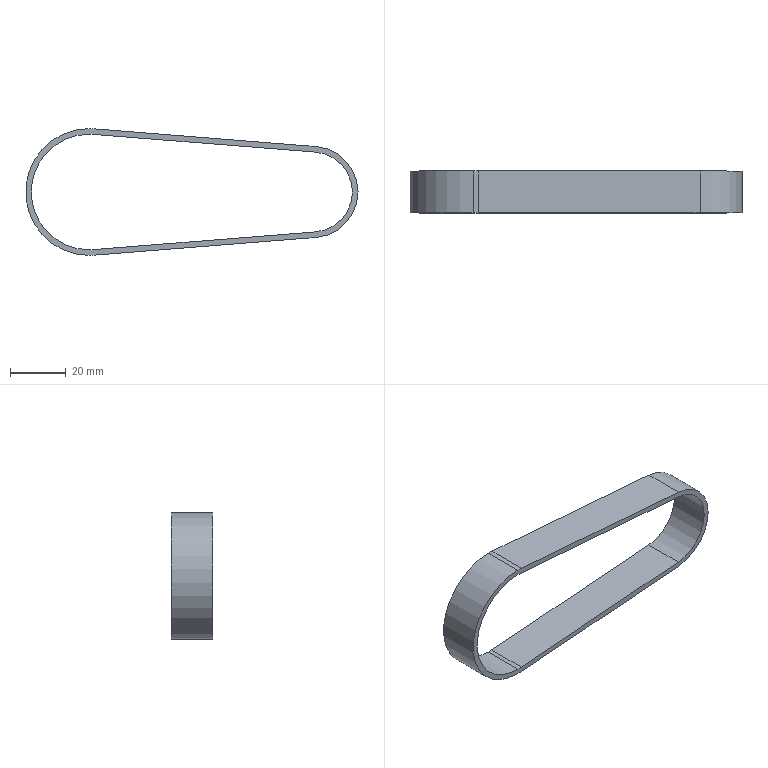Part | STEP file | Timing Belt 270-5M-15mm Wide | 1 solid | 14 faces | box 119.02 x 15 x 45.38 mm | volume 8304 mm3 | cylinder 8 | plane 6 | commonest cylinder face diameters 41.38 x3 45.38 x3 28.66 x1 32.66 x1
STEP:
#1=CARTESIAN_POINT('',(0.,0.,0.));
#2=DIRECTION('',(0.,0.,1.));
#3=DIRECTION('',(1.,0.,0.));
#4=AXIS2_PLACEMENT_3D('',#1,#2,#3);
#5=CARTESIAN_POINT('',(0.,7.5,-20.69));
#6=VERTEX_POINT('',#5);
#7=CARTESIAN_POINT('',(0.,-7.5,-20.69));
#8=VERTEX_POINT('',#7);
#9=CARTESIAN_POINT('',(0.,7.5,-20.69));
#10=DIRECTION('',(0.,-1.,0.));
#11=VECTOR('',#10,1.);
#12=LINE('',#9,#11);
#13=CARTESIAN_POINT('',(0.,7.5,0.));
#14=DIRECTION('',(0.,-1.,0.));
#15=DIRECTION('',(0.,0.,-1.));
#16=AXIS2_PLACEMENT_3D('',#13,#14,#15);
#17=CYLINDRICAL_SURFACE('',#16,20.69);
#18=CARTESIAN_POINT('',(6.283,0.));
#19=DIRECTION('',(0.,1.));
#20=VECTOR('',#19,1.);
#21=LINE('',#18,#20);
#22=(GEOMETRIC_REPRESENTATION_CONTEXT(2)PARAMETRIC_REPRESENTATION_CONTEXT()REPRESENTATION_CONTEXT('',''));
#23=DEFINITIONAL_REPRESENTATION('',(#21),#22);
#24=PCURVE('',#17,#23);
#25=CARTESIAN_POINT('',(0.,7.5,0.));
#26=DIRECTION('',(0.,-1.,0.));
#27=DIRECTION('',(0.,0.,-1.));
#28=AXIS2_PLACEMENT_3D('',#25,#26,#27);
#29=CYLINDRICAL_SURFACE('',#28,20.69);
#30=CARTESIAN_POINT('',(0.,0.));
#31=DIRECTION('',(0.,1.));
#32=VECTOR('',#31,1.);
#33=LINE('',#30,#32);
#34=(GEOMETRIC_REPRESENTATION_CONTEXT(2)PARAMETRIC_REPRESENTATION_CONTEXT()REPRESENTATION_CONTEXT('',''));
#35=DEFINITIONAL_REPRESENTATION('',(#33),#34);
#36=PCURVE('',#29,#35);
#37=SURFACE_CURVE('',#12,(#24,#36),.PCURVE_S1.);
#38=EDGE_CURVE('',#6,#8,#37,.T.);
#39=ORIENTED_EDGE('',*,*,#38,.T.);
#40=CARTESIAN_POINT('',(0.,-7.5,20.69));
#41=VERTEX_POINT('',#40);
#42=CARTESIAN_POINT('',(0.,-7.5,0.));
#43=DIRECTION('',(0.,1.,0.));
#44=DIRECTION('',(0.,0.,1.));
#45=AXIS2_PLACEMENT_3D('',#42,#43,#44);
#46=CIRCLE('',#45,20.69);
#47=CARTESIAN_POINT('',(9.425,15.));
#48=DIRECTION('',(-1.,0.));
#49=VECTOR('',#48,1.);
#50=LINE('',#47,#49);
#51=(GEOMETRIC_REPRESENTATION_CONTEXT(2)PARAMETRIC_REPRESENTATION_CONTEXT()REPRESENTATION_CONTEXT('',''));
#52=DEFINITIONAL_REPRESENTATION('',(#50),#51);
#53=PCURVE('',#17,#52);
#54=CARTESIAN_POINT('',(80.,-7.5,0.));
#55=DIRECTION('',(0.,1.,0.));
#56=DIRECTION('',(0.,0.,1.));
#57=AXIS2_PLACEMENT_3D('',#54,#55,#56);
#58=PLANE('',#57);
#59=CARTESIAN_POINT('',(0.,-80.));
#60=DIRECTION('',(1.,0.));
#61=AXIS2_PLACEMENT_2D('',#59,#60);
#62=CIRCLE('',#61,20.69);
#63=(GEOMETRIC_REPRESENTATION_CONTEXT(2)PARAMETRIC_REPRESENTATION_CONTEXT()REPRESENTATION_CONTEXT('',''));
#64=DEFINITIONAL_REPRESENTATION('',(#62),#63);
#65=PCURVE('',#58,#64);
#66=SURFACE_CURVE('',#46,(#53,#65),.PCURVE_S1.);
#67=EDGE_CURVE('',#8,#41,#66,.T.);
#68=ORIENTED_EDGE('',*,*,#67,.T.);
#69=CARTESIAN_POINT('',(0.,7.5,20.69));
#70=VERTEX_POINT('',#69);
#71=CARTESIAN_POINT('',(0.,7.5,20.69));
#72=DIRECTION('',(0.,-1.,0.));
#73=VECTOR('',#72,1.);
#74=LINE('',#71,#73);
#75=CARTESIAN_POINT('',(3.142,0.));
#76=DIRECTION('',(0.,1.));
#77=VECTOR('',#76,1.);
#78=LINE('',#75,#77);
#79=(GEOMETRIC_REPRESENTATION_CONTEXT(2)PARAMETRIC_REPRESENTATION_CONTEXT()REPRESENTATION_CONTEXT('',''));
#80=DEFINITIONAL_REPRESENTATION('',(#78),#79);
#81=PCURVE('',#17,#80);
#82=CARTESIAN_POINT('',(0.,7.5,0.));
#83=DIRECTION('',(0.,-1.,0.));
#84=DIRECTION('',(0.,0.,-1.));
#85=AXIS2_PLACEMENT_3D('',#82,#83,#84);
#86=CYLINDRICAL_SURFACE('',#85,20.69);
#87=CARTESIAN_POINT('',(3.142,0.));
#88=DIRECTION('',(0.,1.));
#89=VECTOR('',#88,1.);
#90=LINE('',#87,#89);
#91=(GEOMETRIC_REPRESENTATION_CONTEXT(2)PARAMETRIC_REPRESENTATION_CONTEXT()REPRESENTATION_CONTEXT('',''));
#92=DEFINITIONAL_REPRESENTATION('',(#90),#91);
#93=PCURVE('',#86,#92);
#94=SURFACE_CURVE('',#74,(#81,#93),.PCURVE_S1.);
#95=EDGE_CURVE('',#70,#41,#94,.T.);
#96=ORIENTED_EDGE('',*,*,#95,.F.);
#97=CARTESIAN_POINT('',(0.,7.5,0.));
#98=DIRECTION('',(0.,1.,0.));
#99=DIRECTION('',(0.,0.,1.));
#100=AXIS2_PLACEMENT_3D('',#97,#98,#99);
#101=CIRCLE('',#100,20.69);
#102=CARTESIAN_POINT('',(9.425,0.));
#103=DIRECTION('',(-1.,0.));
#104=VECTOR('',#103,1.);
#105=LINE('',#102,#104);
#106=(GEOMETRIC_REPRESENTATION_CONTEXT(2)PARAMETRIC_REPRESENTATION_CONTEXT()REPRESENTATION_CONTEXT('',''));
#107=DEFINITIONAL_REPRESENTATION('',(#105),#106);
#108=PCURVE('',#17,#107);
#109=CARTESIAN_POINT('',(80.,7.5,0.));
#110=DIRECTION('',(0.,1.,0.));
#111=DIRECTION('',(0.,0.,1.));
#112=AXIS2_PLACEMENT_3D('',#109,#110,#111);
#113=PLANE('',#112);
#114=CARTESIAN_POINT('',(0.,-80.));
#115=DIRECTION('',(1.,0.));
#116=AXIS2_PLACEMENT_2D('',#114,#115);
#117=CIRCLE('',#116,20.69);
#118=(GEOMETRIC_REPRESENTATION_CONTEXT(2)PARAMETRIC_REPRESENTATION_CONTEXT()REPRESENTATION_CONTEXT('',''));
#119=DEFINITIONAL_REPRESENTATION('',(#117),#118);
#120=PCURVE('',#113,#119);
#121=SURFACE_CURVE('',#101,(#108,#120),.PCURVE_S1.);
#122=EDGE_CURVE('',#6,#70,#121,.T.);
#123=ORIENTED_EDGE('',*,*,#122,.F.);
#124=EDGE_LOOP('',(#39,#68,#96,#123));
#125=FACE_BOUND('',#124,.F.);
#126=ADVANCED_FACE('',(#125),#17,.F.);
#127=CARTESIAN_POINT('',(1.645,7.5,-20.625));
#128=VERTEX_POINT('',#127);
#129=CARTESIAN_POINT('',(1.645,-7.5,-20.625));
#130=VERTEX_POINT('',#129);
#131=CARTESIAN_POINT('',(1.645,7.5,-20.625));
#132=DIRECTION('',(0.,-1.,0.));
#133=VECTOR('',#132,1.);
#134=LINE('',#131,#133);
#135=CARTESIAN_POINT('',(0.07958,0.));
#136=DIRECTION('',(0.,1.));
#137=VECTOR('',#136,1.);
#138=LINE('',#135,#137);
#139=(GEOMETRIC_REPRESENTATION_CONTEXT(2)PARAMETRIC_REPRESENTATION_CONTEXT()REPRESENTATION_CONTEXT('',''));
#140=DEFINITIONAL_REPRESENTATION('',(#138),#139);
#141=PCURVE('',#29,#140);
#142=CARTESIAN_POINT('',(1.645,7.5,-20.625));
#143=DIRECTION('',(-0.0795,0.,0.9968));
#144=DIRECTION('',(0.9968,0.,0.0795));
#145=AXIS2_PLACEMENT_3D('',#142,#143,#144);
#146=PLANE('',#145);
#147=CARTESIAN_POINT('',(0.,0.));
#148=DIRECTION('',(0.,-1.));
#149=VECTOR('',#148,1.);
#150=LINE('',#147,#149);
#151=(GEOMETRIC_REPRESENTATION_CONTEXT(2)PARAMETRIC_REPRESENTATION_CONTEXT()REPRESENTATION_CONTEXT('',''));
#152=DEFINITIONAL_REPRESENTATION('',(#150),#151);
#153=PCURVE('',#146,#152);
#154=SURFACE_CURVE('',#134,(#141,#153),.PCURVE_S1.);
#155=EDGE_CURVE('',#128,#130,#154,.T.);
#156=ORIENTED_EDGE('',*,*,#155,.T.);
#157=CARTESIAN_POINT('',(0.,-7.5,0.));
#158=DIRECTION('',(0.,1.,0.));
#159=DIRECTION('',(0.,0.,1.));
#160=AXIS2_PLACEMENT_3D('',#157,#158,#159);
#161=CIRCLE('',#160,20.69);
#162=CARTESIAN_POINT('',(3.142,15.));
#163=DIRECTION('',(-1.,0.));
#164=VECTOR('',#163,1.);
#165=LINE('',#162,#164);
#166=(GEOMETRIC_REPRESENTATION_CONTEXT(2)PARAMETRIC_REPRESENTATION_CONTEXT()REPRESENTATION_CONTEXT('',''));
#167=DEFINITIONAL_REPRESENTATION('',(#165),#166);
#168=PCURVE('',#29,#167);
#169=CARTESIAN_POINT('',(0.,-80.));
#170=DIRECTION('',(1.,0.));
#171=AXIS2_PLACEMENT_2D('',#169,#170);
#172=CIRCLE('',#171,20.69);
#173=(GEOMETRIC_REPRESENTATION_CONTEXT(2)PARAMETRIC_REPRESENTATION_CONTEXT()REPRESENTATION_CONTEXT('',''));
#174=DEFINITIONAL_REPRESENTATION('',(#172),#173);
#175=PCURVE('',#58,#174);
#176=SURFACE_CURVE('',#161,(#168,#175),.PCURVE_S1.);
#177=EDGE_CURVE('',#130,#8,#176,.T.);
#178=ORIENTED_EDGE('',*,*,#177,.T.);
#179=ORIENTED_EDGE('',*,*,#38,.F.);
#180=CARTESIAN_POINT('',(0.,7.5,0.));
#181=DIRECTION('',(0.,1.,0.));
#182=DIRECTION('',(0.,0.,1.));
#183=AXIS2_PLACEMENT_3D('',#180,#181,#182);
#184=CIRCLE('',#183,20.69);
#185=CARTESIAN_POINT('',(3.142,0.));
#186=DIRECTION('',(-1.,0.));
#187=VECTOR('',#186,1.);
#188=LINE('',#185,#187);
#189=(GEOMETRIC_REPRESENTATION_CONTEXT(2)PARAMETRIC_REPRESENTATION_CONTEXT()REPRESENTATION_CONTEXT('',''));
#190=DEFINITIONAL_REPRESENTATION('',(#188),#189);
#191=PCURVE('',#29,#190);
#192=CARTESIAN_POINT('',(0.,-80.));
#193=DIRECTION('',(1.,0.));
#194=AXIS2_PLACEMENT_2D('',#192,#193);
#195=CIRCLE('',#194,20.69);
#196=(GEOMETRIC_REPRESENTATION_CONTEXT(2)PARAMETRIC_REPRESENTATION_CONTEXT()REPRESENTATION_CONTEXT('',''));
#197=DEFINITIONAL_REPRESENTATION('',(#195),#196);
#198=PCURVE('',#113,#197);
#199=SURFACE_CURVE('',#184,(#191,#198),.PCURVE_S1.);
#200=EDGE_CURVE('',#128,#6,#199,.T.);
#201=ORIENTED_EDGE('',*,*,#200,.F.);
#202=EDGE_LOOP('',(#156,#178,#179,#201));
#203=FACE_BOUND('',#202,.F.);
#204=ADVANCED_FACE('',(#203),#29,.F.);
#205=CARTESIAN_POINT('',(0.,7.5,22.69));
#206=VERTEX_POINT('',#205);
#207=CARTESIAN_POINT('',(1.804,7.5,22.618));
#208=VERTEX_POINT('',#207);
#209=CARTESIAN_POINT('',(0.,7.5,0.));
#210=DIRECTION('',(0.,1.,0.));
#211=DIRECTION('',(1.,0.,0.));
#212=AXIS2_PLACEMENT_3D('',#209,#210,#211);
#213=CIRCLE('',#212,22.69);
#214=CARTESIAN_POINT('',(0.,7.5,0.));
#215=DIRECTION('',(0.,-1.,0.));
#216=DIRECTION('',(0.,0.,-1.));
#217=AXIS2_PLACEMENT_3D('',#214,#215,#216);
#218=CYLINDRICAL_SURFACE('',#217,22.69);
#219=CARTESIAN_POINT('',(7.854,0.));
#220=DIRECTION('',(-1.,0.));
#221=VECTOR('',#220,1.);
#222=LINE('',#219,#221);
#223=(GEOMETRIC_REPRESENTATION_CONTEXT(2)PARAMETRIC_REPRESENTATION_CONTEXT()REPRESENTATION_CONTEXT('',''));
#224=DEFINITIONAL_REPRESENTATION('',(#222),#223);
#225=PCURVE('',#218,#224);
#226=CARTESIAN_POINT('',(0.,-80.));
#227=DIRECTION('',(0.,1.));
#228=AXIS2_PLACEMENT_2D('',#226,#227);
#229=CIRCLE('',#228,22.69);
#230=(GEOMETRIC_REPRESENTATION_CONTEXT(2)PARAMETRIC_REPRESENTATION_CONTEXT()REPRESENTATION_CONTEXT('',''));
#231=DEFINITIONAL_REPRESENTATION('',(#229),#230);
#232=PCURVE('',#113,#231);
#233=SURFACE_CURVE('',#213,(#225,#232),.PCURVE_S1.);
#234=EDGE_CURVE('',#206,#208,#233,.T.);
#235=ORIENTED_EDGE('',*,*,#234,.F.);
#236=CARTESIAN_POINT('',(0.,-7.5,22.69));
#237=VERTEX_POINT('',#236);
#238=CARTESIAN_POINT('',(0.,7.5,22.69));
#239=DIRECTION('',(0.,-1.,0.));
#240=VECTOR('',#239,1.);
#241=LINE('',#238,#240);
#242=CARTESIAN_POINT('',(3.142,0.));
#243=DIRECTION('',(0.,1.));
#244=VECTOR('',#243,1.);
#245=LINE('',#242,#244);
#246=(GEOMETRIC_REPRESENTATION_CONTEXT(2)PARAMETRIC_REPRESENTATION_CONTEXT()REPRESENTATION_CONTEXT('',''));
#247=DEFINITIONAL_REPRESENTATION('',(#245),#246);
#248=PCURVE('',#218,#247);
#249=CARTESIAN_POINT('',(0.,7.5,0.));
#250=DIRECTION('',(0.,-1.,0.));
#251=DIRECTION('',(0.,0.,-1.));
#252=AXIS2_PLACEMENT_3D('',#249,#250,#251);
#253=CYLINDRICAL_SURFACE('',#252,22.69);
#254=CARTESIAN_POINT('',(3.142,0.));
#255=DIRECTION('',(0.,1.));
#256=VECTOR('',#255,1.);
#257=LINE('',#254,#256);
#258=(GEOMETRIC_REPRESENTATION_CONTEXT(2)PARAMETRIC_REPRESENTATION_CONTEXT()REPRESENTATION_CONTEXT('',''));
#259=DEFINITIONAL_REPRESENTATION('',(#257),#258);
#260=PCURVE('',#253,#259);
#261=SURFACE_CURVE('',#241,(#248,#260),.PCURVE_S1.);
#262=EDGE_CURVE('',#206,#237,#261,.T.);
#263=ORIENTED_EDGE('',*,*,#262,.T.);
#264=CARTESIAN_POINT('',(1.804,-7.5,22.618));
#265=VERTEX_POINT('',#264);
#266=CARTESIAN_POINT('',(0.,-7.5,0.));
#267=DIRECTION('',(0.,1.,0.));
#268=DIRECTION('',(1.,0.,0.));
#269=AXIS2_PLACEMENT_3D('',#266,#267,#268);
#270=CIRCLE('',#269,22.69);
#271=CARTESIAN_POINT('',(7.854,15.));
#272=DIRECTION('',(-1.,0.));
#273=VECTOR('',#272,1.);
#274=LINE('',#271,#273);
#275=(GEOMETRIC_REPRESENTATION_CONTEXT(2)PARAMETRIC_REPRESENTATION_CONTEXT()REPRESENTATION_CONTEXT('',''));
#276=DEFINITIONAL_REPRESENTATION('',(#274),#275);
#277=PCURVE('',#218,#276);
#278=CARTESIAN_POINT('',(0.,-80.));
#279=DIRECTION('',(0.,1.));
#280=AXIS2_PLACEMENT_2D('',#278,#279);
#281=CIRCLE('',#280,22.69);
#282=(GEOMETRIC_REPRESENTATION_CONTEXT(2)PARAMETRIC_REPRESENTATION_CONTEXT()REPRESENTATION_CONTEXT('',''));
#283=DEFINITIONAL_REPRESENTATION('',(#281),#282);
#284=PCURVE('',#58,#283);
#285=SURFACE_CURVE('',#270,(#277,#284),.PCURVE_S1.);
#286=EDGE_CURVE('',#237,#265,#285,.T.);
#287=ORIENTED_EDGE('',*,*,#286,.T.);
#288=CARTESIAN_POINT('',(1.804,7.5,22.618));
#289=DIRECTION('',(0.,-1.,0.));
#290=VECTOR('',#289,1.);
#291=LINE('',#288,#290);
#292=CARTESIAN_POINT('',(3.062,0.));
#293=DIRECTION('',(0.,1.));
#294=VECTOR('',#293,1.);
#295=LINE('',#292,#294);
#296=(GEOMETRIC_REPRESENTATION_CONTEXT(2)PARAMETRIC_REPRESENTATION_CONTEXT()REPRESENTATION_CONTEXT('',''));
#297=DEFINITIONAL_REPRESENTATION('',(#295),#296);
#298=PCURVE('',#218,#297);
#299=CARTESIAN_POINT('',(1.804,7.5,22.618));
#300=DIRECTION('',(-0.0795,0.,-0.9968));
#301=DIRECTION('',(-0.9968,0.,0.0795));
#302=AXIS2_PLACEMENT_3D('',#299,#300,#301);
#303=PLANE('',#302);
#304=CARTESIAN_POINT('',(0.,0.));
#305=DIRECTION('',(0.,-1.));
#306=VECTOR('',#305,1.);
#307=LINE('',#304,#306);
#308=(GEOMETRIC_REPRESENTATION_CONTEXT(2)PARAMETRIC_REPRESENTATION_CONTEXT()REPRESENTATION_CONTEXT('',''));
#309=DEFINITIONAL_REPRESENTATION('',(#307),#308);
#310=PCURVE('',#303,#309);
#311=SURFACE_CURVE('',#291,(#298,#310),.PCURVE_S1.);
#312=EDGE_CURVE('',#208,#265,#311,.T.);
#313=ORIENTED_EDGE('',*,*,#312,.F.);
#314=EDGE_LOOP('',(#235,#263,#287,#313));
#315=FACE_BOUND('',#314,.T.);
#316=ADVANCED_FACE('',(#315),#218,.T.);
#317=ORIENTED_EDGE('',*,*,#262,.F.);
#318=CARTESIAN_POINT('',(0.,7.5,-22.69));
#319=VERTEX_POINT('',#318);
#320=CARTESIAN_POINT('',(0.,7.5,0.));
#321=DIRECTION('',(0.,1.,0.));
#322=DIRECTION('',(1.,0.,0.));
#323=AXIS2_PLACEMENT_3D('',#320,#321,#322);
#324=CIRCLE('',#323,22.69);
#325=CARTESIAN_POINT('',(7.854,0.));
#326=DIRECTION('',(-1.,0.));
#327=VECTOR('',#326,1.);
#328=LINE('',#325,#327);
#329=(GEOMETRIC_REPRESENTATION_CONTEXT(2)PARAMETRIC_REPRESENTATION_CONTEXT()REPRESENTATION_CONTEXT('',''));
#330=DEFINITIONAL_REPRESENTATION('',(#328),#329);
#331=PCURVE('',#253,#330);
#332=CARTESIAN_POINT('',(0.,-80.));
#333=DIRECTION('',(0.,1.));
#334=AXIS2_PLACEMENT_2D('',#332,#333);
#335=CIRCLE('',#334,22.69);
#336=(GEOMETRIC_REPRESENTATION_CONTEXT(2)PARAMETRIC_REPRESENTATION_CONTEXT()REPRESENTATION_CONTEXT('',''));
#337=DEFINITIONAL_REPRESENTATION('',(#335),#336);
#338=PCURVE('',#113,#337);
#339=SURFACE_CURVE('',#324,(#331,#338),.PCURVE_S1.);
#340=EDGE_CURVE('',#319,#206,#339,.T.);
#341=ORIENTED_EDGE('',*,*,#340,.F.);
#342=CARTESIAN_POINT('',(0.,-7.5,-22.69));
#343=VERTEX_POINT('',#342);
#344=CARTESIAN_POINT('',(0.,7.5,-22.69));
#345=DIRECTION('',(0.,-1.,0.));
#346=VECTOR('',#345,1.);
#347=LINE('',#344,#346);
#348=CARTESIAN_POINT('',(6.283,0.));
#349=DIRECTION('',(0.,1.));
#350=VECTOR('',#349,1.);
#351=LINE('',#348,#350);
#352=(GEOMETRIC_REPRESENTATION_CONTEXT(2)PARAMETRIC_REPRESENTATION_CONTEXT()REPRESENTATION_CONTEXT('',''));
#353=DEFINITIONAL_REPRESENTATION('',(#351),#352);
#354=PCURVE('',#253,#353);
#355=CARTESIAN_POINT('',(0.,7.5,0.));
#356=DIRECTION('',(0.,-1.,0.));
#357=DIRECTION('',(0.,0.,-1.));
#358=AXIS2_PLACEMENT_3D('',#355,#356,#357);
#359=CYLINDRICAL_SURFACE('',#358,22.69);
#360=CARTESIAN_POINT('',(0.,0.));
#361=DIRECTION('',(0.,1.));
#362=VECTOR('',#361,1.);
#363=LINE('',#360,#362);
#364=(GEOMETRIC_REPRESENTATION_CONTEXT(2)PARAMETRIC_REPRESENTATION_CONTEXT()REPRESENTATION_CONTEXT('',''));
#365=DEFINITIONAL_REPRESENTATION('',(#363),#364);
#366=PCURVE('',#359,#365);
#367=SURFACE_CURVE('',#347,(#354,#366),.PCURVE_S1.);
#368=EDGE_CURVE('',#319,#343,#367,.T.);
#369=ORIENTED_EDGE('',*,*,#368,.T.);
#370=CARTESIAN_POINT('',(0.,-7.5,0.));
#371=DIRECTION('',(0.,1.,0.));
#372=DIRECTION('',(1.,0.,0.));
#373=AXIS2_PLACEMENT_3D('',#370,#371,#372);
#374=CIRCLE('',#373,22.69);
#375=CARTESIAN_POINT('',(7.854,15.));
#376=DIRECTION('',(-1.,0.));
#377=VECTOR('',#376,1.);
#378=LINE('',#375,#377);
#379=(GEOMETRIC_REPRESENTATION_CONTEXT(2)PARAMETRIC_REPRESENTATION_CONTEXT()REPRESENTATION_CONTEXT('',''));
#380=DEFINITIONAL_REPRESENTATION('',(#378),#379);
#381=PCURVE('',#253,#380);
#382=CARTESIAN_POINT('',(0.,-80.));
#383=DIRECTION('',(0.,1.));
#384=AXIS2_PLACEMENT_2D('',#382,#383);
#385=CIRCLE('',#384,22.69);
#386=(GEOMETRIC_REPRESENTATION_CONTEXT(2)PARAMETRIC_REPRESENTATION_CONTEXT()REPRESENTATION_CONTEXT('',''));
#387=DEFINITIONAL_REPRESENTATION('',(#385),#386);
#388=PCURVE('',#58,#387);
#389=SURFACE_CURVE('',#374,(#381,#388),.PCURVE_S1.);
#390=EDGE_CURVE('',#343,#237,#389,.T.);
#391=ORIENTED_EDGE('',*,*,#390,.T.);
#392=EDGE_LOOP('',(#317,#341,#369,#391));
#393=FACE_BOUND('',#392,.T.);
#394=ADVANCED_FACE('',(#393),#253,.T.);
#395=CARTESIAN_POINT('',(81.298,7.5,16.278));
#396=VERTEX_POINT('',#395);
#397=CARTESIAN_POINT('',(81.298,7.5,-16.278));
#398=VERTEX_POINT('',#397);
#399=CARTESIAN_POINT('',(80.,7.5,0.));
#400=DIRECTION('',(0.,1.,0.));
#401=DIRECTION('',(1.,0.,0.));
#402=AXIS2_PLACEMENT_3D('',#399,#400,#401);
#403=CIRCLE('',#402,16.33);
#404=CARTESIAN_POINT('',(0.,0.));
#405=DIRECTION('',(0.,1.));
#406=AXIS2_PLACEMENT_2D('',#404,#405);
#407=CIRCLE('',#406,16.33);
#408=(GEOMETRIC_REPRESENTATION_CONTEXT(2)PARAMETRIC_REPRESENTATION_CONTEXT()REPRESENTATION_CONTEXT('',''));
#409=DEFINITIONAL_REPRESENTATION('',(#407),#408);
#410=PCURVE('',#113,#409);
#411=CARTESIAN_POINT('',(80.,7.5,0.));
#412=DIRECTION('',(0.,-1.,0.));
#413=DIRECTION('',(0.,0.,-1.));
#414=AXIS2_PLACEMENT_3D('',#411,#412,#413);
#415=CYLINDRICAL_SURFACE('',#414,16.33);
#416=CARTESIAN_POINT('',(7.854,0.));
#417=DIRECTION('',(-1.,0.));
#418=VECTOR('',#417,1.);
#419=LINE('',#416,#418);
#420=(GEOMETRIC_REPRESENTATION_CONTEXT(2)PARAMETRIC_REPRESENTATION_CONTEXT()REPRESENTATION_CONTEXT('',''));
#421=DEFINITIONAL_REPRESENTATION('',(#419),#420);
#422=PCURVE('',#415,#421);
#423=SURFACE_CURVE('',#403,(#410,#422),.PCURVE_S1.);
#424=EDGE_CURVE('',#396,#398,#423,.T.);
#425=ORIENTED_EDGE('',*,*,#424,.T.);
#426=CARTESIAN_POINT('',(1.804,7.5,-22.618));
#427=VERTEX_POINT('',#426);
#428=CARTESIAN_POINT('',(1.804,7.5,-22.618));
#429=DIRECTION('',(-0.9968,0.,-0.0795));
#430=VECTOR('',#429,1.);
#431=LINE('',#428,#430);
#432=CARTESIAN_POINT('',(-22.618,-78.196));
#433=DIRECTION('',(-0.0795,-0.9968));
#434=VECTOR('',#433,1.);
#435=LINE('',#432,#434);
#436=(GEOMETRIC_REPRESENTATION_CONTEXT(2)PARAMETRIC_REPRESENTATION_CONTEXT()REPRESENTATION_CONTEXT('',''));
#437=DEFINITIONAL_REPRESENTATION('',(#435),#436);
#438=PCURVE('',#113,#437);
#439=CARTESIAN_POINT('',(1.804,7.5,-22.618));
#440=DIRECTION('',(-0.0795,0.,0.9968));
#441=DIRECTION('',(0.9968,0.,0.0795));
#442=AXIS2_PLACEMENT_3D('',#439,#440,#441);
#443=PLANE('',#442);
#444=CARTESIAN_POINT('',(0.,0.));
#445=DIRECTION('',(-1.,0.));
#446=VECTOR('',#445,1.);
#447=LINE('',#444,#446);
#448=(GEOMETRIC_REPRESENTATION_CONTEXT(2)PARAMETRIC_REPRESENTATION_CONTEXT()REPRESENTATION_CONTEXT('',''));
#449=DEFINITIONAL_REPRESENTATION('',(#447),#448);
#450=PCURVE('',#443,#449);
#451=SURFACE_CURVE('',#431,(#438,#450),.PCURVE_S1.);
#452=EDGE_CURVE('',#398,#427,#451,.T.);
#453=ORIENTED_EDGE('',*,*,#452,.T.);
#454=CARTESIAN_POINT('',(0.,7.5,0.));
#455=DIRECTION('',(0.,1.,0.));
#456=DIRECTION('',(1.,0.,0.));
#457=AXIS2_PLACEMENT_3D('',#454,#455,#456);
#458=CIRCLE('',#457,22.69);
#459=CARTESIAN_POINT('',(0.,-80.));
#460=DIRECTION('',(0.,1.));
#461=AXIS2_PLACEMENT_2D('',#459,#460);
#462=CIRCLE('',#461,22.69);
#463=(GEOMETRIC_REPRESENTATION_CONTEXT(2)PARAMETRIC_REPRESENTATION_CONTEXT()REPRESENTATION_CONTEXT('',''));
#464=DEFINITIONAL_REPRESENTATION('',(#462),#463);
#465=PCURVE('',#113,#464);
#466=CARTESIAN_POINT('',(1.571,0.));
#467=DIRECTION('',(-1.,0.));
#468=VECTOR('',#467,1.);
#469=LINE('',#466,#468);
#470=(GEOMETRIC_REPRESENTATION_CONTEXT(2)PARAMETRIC_REPRESENTATION_CONTEXT()REPRESENTATION_CONTEXT('',''));
#471=DEFINITIONAL_REPRESENTATION('',(#469),#470);
#472=PCURVE('',#359,#471);
#473=SURFACE_CURVE('',#458,(#465,#472),.PCURVE_S1.);
#474=EDGE_CURVE('',#427,#319,#473,.T.);
#475=ORIENTED_EDGE('',*,*,#474,.T.);
#476=ORIENTED_EDGE('',*,*,#340,.T.);
#477=ORIENTED_EDGE('',*,*,#234,.T.);
#478=CARTESIAN_POINT('',(1.804,7.5,22.618));
#479=DIRECTION('',(0.9968,0.,-0.0795));
#480=VECTOR('',#479,1.);
#481=LINE('',#478,#480);
#482=CARTESIAN_POINT('',(22.618,-78.196));
#483=DIRECTION('',(-0.0795,0.9968));
#484=VECTOR('',#483,1.);
#485=LINE('',#482,#484);
#486=(GEOMETRIC_REPRESENTATION_CONTEXT(2)PARAMETRIC_REPRESENTATION_CONTEXT()REPRESENTATION_CONTEXT('',''));
#487=DEFINITIONAL_REPRESENTATION('',(#485),#486);
#488=PCURVE('',#113,#487);
#489=CARTESIAN_POINT('',(0.,0.));
#490=DIRECTION('',(-1.,0.));
#491=VECTOR('',#490,1.);
#492=LINE('',#489,#491);
#493=(GEOMETRIC_REPRESENTATION_CONTEXT(2)PARAMETRIC_REPRESENTATION_CONTEXT()REPRESENTATION_CONTEXT('',''));
#494=DEFINITIONAL_REPRESENTATION('',(#492),#493);
#495=PCURVE('',#303,#494);
#496=SURFACE_CURVE('',#481,(#488,#495),.PCURVE_S1.);
#497=EDGE_CURVE('',#208,#396,#496,.T.);
#498=ORIENTED_EDGE('',*,*,#497,.T.);
#499=EDGE_LOOP('',(#425,#453,#475,#476,#477,#498));
#500=FACE_BOUND('',#499,.T.);
#501=CARTESIAN_POINT('',(81.139,7.5,-14.285));
#502=VERTEX_POINT('',#501);
#503=CARTESIAN_POINT('',(1.645,7.5,-20.625));
#504=DIRECTION('',(-0.9968,0.,-0.0795));
#505=VECTOR('',#504,1.);
#506=LINE('',#503,#505);
#507=CARTESIAN_POINT('',(-20.625,-78.355));
#508=DIRECTION('',(-0.0795,-0.9968));
#509=VECTOR('',#508,1.);
#510=LINE('',#507,#509);
#511=(GEOMETRIC_REPRESENTATION_CONTEXT(2)PARAMETRIC_REPRESENTATION_CONTEXT()REPRESENTATION_CONTEXT('',''));
#512=DEFINITIONAL_REPRESENTATION('',(#510),#511);
#513=PCURVE('',#113,#512);
#514=CARTESIAN_POINT('',(0.,0.));
#515=DIRECTION('',(-1.,0.));
#516=VECTOR('',#515,1.);
#517=LINE('',#514,#516);
#518=(GEOMETRIC_REPRESENTATION_CONTEXT(2)PARAMETRIC_REPRESENTATION_CONTEXT()REPRESENTATION_CONTEXT('',''));
#519=DEFINITIONAL_REPRESENTATION('',(#517),#518);
#520=PCURVE('',#146,#519);
#521=SURFACE_CURVE('',#506,(#513,#520),.PCURVE_S1.);
#522=EDGE_CURVE('',#502,#128,#521,.T.);
#523=ORIENTED_EDGE('',*,*,#522,.F.);
#524=CARTESIAN_POINT('',(81.139,7.5,14.285));
#525=VERTEX_POINT('',#524);
#526=CARTESIAN_POINT('',(80.,7.5,0.));
#527=DIRECTION('',(0.,1.,0.));
#528=DIRECTION('',(0.,0.,1.));
#529=AXIS2_PLACEMENT_3D('',#526,#527,#528);
#530=CIRCLE('',#529,14.33);
#531=CARTESIAN_POINT('',(0.,0.));
#532=DIRECTION('',(1.,0.));
#533=AXIS2_PLACEMENT_2D('',#531,#532);
#534=CIRCLE('',#533,14.33);
#535=(GEOMETRIC_REPRESENTATION_CONTEXT(2)PARAMETRIC_REPRESENTATION_CONTEXT()REPRESENTATION_CONTEXT('',''));
#536=DEFINITIONAL_REPRESENTATION('',(#534),#535);
#537=PCURVE('',#113,#536);
#538=CARTESIAN_POINT('',(80.,7.5,0.));
#539=DIRECTION('',(0.,-1.,0.));
#540=DIRECTION('',(0.,0.,-1.));
#541=AXIS2_PLACEMENT_3D('',#538,#539,#540);
#542=CYLINDRICAL_SURFACE('',#541,14.33);
#543=CARTESIAN_POINT('',(3.142,0.));
#544=DIRECTION('',(-1.,0.));
#545=VECTOR('',#544,1.);
#546=LINE('',#543,#545);
#547=(GEOMETRIC_REPRESENTATION_CONTEXT(2)PARAMETRIC_REPRESENTATION_CONTEXT()REPRESENTATION_CONTEXT('',''));
#548=DEFINITIONAL_REPRESENTATION('',(#546),#547);
#549=PCURVE('',#542,#548);
#550=SURFACE_CURVE('',#530,(#537,#549),.PCURVE_S1.);
#551=EDGE_CURVE('',#525,#502,#550,.T.);
#552=ORIENTED_EDGE('',*,*,#551,.F.);
#553=CARTESIAN_POINT('',(1.645,7.5,20.625));
#554=VERTEX_POINT('',#553);
#555=CARTESIAN_POINT('',(1.645,7.5,20.625));
#556=DIRECTION('',(0.9968,0.,-0.0795));
#557=VECTOR('',#556,1.);
#558=LINE('',#555,#557);
#559=CARTESIAN_POINT('',(20.625,-78.355));
#560=DIRECTION('',(-0.0795,0.9968));
#561=VECTOR('',#560,1.);
#562=LINE('',#559,#561);
#563=(GEOMETRIC_REPRESENTATION_CONTEXT(2)PARAMETRIC_REPRESENTATION_CONTEXT()REPRESENTATION_CONTEXT('',''));
#564=DEFINITIONAL_REPRESENTATION('',(#562),#563);
#565=PCURVE('',#113,#564);
#566=CARTESIAN_POINT('',(1.645,7.5,20.625));
#567=DIRECTION('',(-0.0795,0.,-0.9968));
#568=DIRECTION('',(-0.9968,0.,0.0795));
#569=AXIS2_PLACEMENT_3D('',#566,#567,#568);
#570=PLANE('',#569);
#571=CARTESIAN_POINT('',(0.,0.));
#572=DIRECTION('',(-1.,0.));
#573=VECTOR('',#572,1.);
#574=LINE('',#571,#573);
#575=(GEOMETRIC_REPRESENTATION_CONTEXT(2)PARAMETRIC_REPRESENTATION_CONTEXT()REPRESENTATION_CONTEXT('',''));
#576=DEFINITIONAL_REPRESENTATION('',(#574),#575);
#577=PCURVE('',#570,#576);
#578=SURFACE_CURVE('',#558,(#565,#577),.PCURVE_S1.);
#579=EDGE_CURVE('',#554,#525,#578,.T.);
#580=ORIENTED_EDGE('',*,*,#579,.F.);
#581=CARTESIAN_POINT('',(0.,7.5,0.));
#582=DIRECTION('',(0.,1.,0.));
#583=DIRECTION('',(0.,0.,1.));
#584=AXIS2_PLACEMENT_3D('',#581,#582,#583);
#585=CIRCLE('',#584,20.69);
#586=CARTESIAN_POINT('',(0.,-80.));
#587=DIRECTION('',(1.,0.));
#588=AXIS2_PLACEMENT_2D('',#586,#587);
#589=CIRCLE('',#588,20.69);
#590=(GEOMETRIC_REPRESENTATION_CONTEXT(2)PARAMETRIC_REPRESENTATION_CONTEXT()REPRESENTATION_CONTEXT('',''));
#591=DEFINITIONAL_REPRESENTATION('',(#589),#590);
#592=PCURVE('',#113,#591);
#593=CARTESIAN_POINT('',(3.142,0.));
#594=DIRECTION('',(-1.,0.));
#595=VECTOR('',#594,1.);
#596=LINE('',#593,#595);
#597=(GEOMETRIC_REPRESENTATION_CONTEXT(2)PARAMETRIC_REPRESENTATION_CONTEXT()REPRESENTATION_CONTEXT('',''));
#598=DEFINITIONAL_REPRESENTATION('',(#596),#597);
#599=PCURVE('',#86,#598);
#600=SURFACE_CURVE('',#585,(#592,#599),.PCURVE_S1.);
#601=EDGE_CURVE('',#70,#554,#600,.T.);
#602=ORIENTED_EDGE('',*,*,#601,.F.);
#603=ORIENTED_EDGE('',*,*,#122,.F.);
#604=ORIENTED_EDGE('',*,*,#200,.F.);
#605=EDGE_LOOP('',(#523,#552,#580,#602,#603,#604));
#606=FACE_BOUND('',#605,.T.);
#607=ADVANCED_FACE('',(#500,#606),#113,.T.);
#608=CARTESIAN_POINT('',(81.298,-7.5,16.278));
#609=VERTEX_POINT('',#608);
#610=CARTESIAN_POINT('',(81.298,-7.5,-16.278));
#611=VERTEX_POINT('',#610);
#612=CARTESIAN_POINT('',(80.,-7.5,0.));
#613=DIRECTION('',(0.,1.,0.));
#614=DIRECTION('',(1.,0.,0.));
#615=AXIS2_PLACEMENT_3D('',#612,#613,#614);
#616=CIRCLE('',#615,16.33);
#617=CARTESIAN_POINT('',(0.,0.));
#618=DIRECTION('',(0.,1.));
#619=AXIS2_PLACEMENT_2D('',#617,#618);
#620=CIRCLE('',#619,16.33);
#621=(GEOMETRIC_REPRESENTATION_CONTEXT(2)PARAMETRIC_REPRESENTATION_CONTEXT()REPRESENTATION_CONTEXT('',''));
#622=DEFINITIONAL_REPRESENTATION('',(#620),#621);
#623=PCURVE('',#58,#622);
#624=CARTESIAN_POINT('',(7.854,15.));
#625=DIRECTION('',(-1.,0.));
#626=VECTOR('',#625,1.);
#627=LINE('',#624,#626);
#628=(GEOMETRIC_REPRESENTATION_CONTEXT(2)PARAMETRIC_REPRESENTATION_CONTEXT()REPRESENTATION_CONTEXT('',''));
#629=DEFINITIONAL_REPRESENTATION('',(#627),#628);
#630=PCURVE('',#415,#629);
#631=SURFACE_CURVE('',#616,(#623,#630),.PCURVE_S1.);
#632=EDGE_CURVE('',#609,#611,#631,.T.);
#633=ORIENTED_EDGE('',*,*,#632,.F.);
#634=CARTESIAN_POINT('',(1.804,-7.5,22.618));
#635=DIRECTION('',(0.9968,0.,-0.0795));
#636=VECTOR('',#635,1.);
#637=LINE('',#634,#636);
#638=CARTESIAN_POINT('',(22.618,-78.196));
#639=DIRECTION('',(-0.0795,0.9968));
#640=VECTOR('',#639,1.);
#641=LINE('',#638,#640);
#642=(GEOMETRIC_REPRESENTATION_CONTEXT(2)PARAMETRIC_REPRESENTATION_CONTEXT()REPRESENTATION_CONTEXT('',''));
#643=DEFINITIONAL_REPRESENTATION('',(#641),#642);
#644=PCURVE('',#58,#643);
#645=CARTESIAN_POINT('',(0.,-15.));
#646=DIRECTION('',(-1.,0.));
#647=VECTOR('',#646,1.);
#648=LINE('',#645,#647);
#649=(GEOMETRIC_REPRESENTATION_CONTEXT(2)PARAMETRIC_REPRESENTATION_CONTEXT()REPRESENTATION_CONTEXT('',''));
#650=DEFINITIONAL_REPRESENTATION('',(#648),#649);
#651=PCURVE('',#303,#650);
#652=SURFACE_CURVE('',#637,(#644,#651),.PCURVE_S1.);
#653=EDGE_CURVE('',#265,#609,#652,.T.);
#654=ORIENTED_EDGE('',*,*,#653,.F.);
#655=ORIENTED_EDGE('',*,*,#286,.F.);
#656=ORIENTED_EDGE('',*,*,#390,.F.);
#657=CARTESIAN_POINT('',(1.804,-7.5,-22.618));
#658=VERTEX_POINT('',#657);
#659=CARTESIAN_POINT('',(0.,-7.5,0.));
#660=DIRECTION('',(0.,1.,0.));
#661=DIRECTION('',(1.,0.,0.));
#662=AXIS2_PLACEMENT_3D('',#659,#660,#661);
#663=CIRCLE('',#662,22.69);
#664=CARTESIAN_POINT('',(0.,-80.));
#665=DIRECTION('',(0.,1.));
#666=AXIS2_PLACEMENT_2D('',#664,#665);
#667=CIRCLE('',#666,22.69);
#668=(GEOMETRIC_REPRESENTATION_CONTEXT(2)PARAMETRIC_REPRESENTATION_CONTEXT()REPRESENTATION_CONTEXT('',''));
#669=DEFINITIONAL_REPRESENTATION('',(#667),#668);
#670=PCURVE('',#58,#669);
#671=CARTESIAN_POINT('',(1.571,15.));
#672=DIRECTION('',(-1.,0.));
#673=VECTOR('',#672,1.);
#674=LINE('',#671,#673);
#675=(GEOMETRIC_REPRESENTATION_CONTEXT(2)PARAMETRIC_REPRESENTATION_CONTEXT()REPRESENTATION_CONTEXT('',''));
#676=DEFINITIONAL_REPRESENTATION('',(#674),#675);
#677=PCURVE('',#359,#676);
#678=SURFACE_CURVE('',#663,(#670,#677),.PCURVE_S1.);
#679=EDGE_CURVE('',#658,#343,#678,.T.);
#680=ORIENTED_EDGE('',*,*,#679,.F.);
#681=CARTESIAN_POINT('',(1.804,-7.5,-22.618));
#682=DIRECTION('',(-0.9968,0.,-0.0795));
#683=VECTOR('',#682,1.);
#684=LINE('',#681,#683);
#685=CARTESIAN_POINT('',(-22.618,-78.196));
#686=DIRECTION('',(-0.0795,-0.9968));
#687=VECTOR('',#686,1.);
#688=LINE('',#685,#687);
#689=(GEOMETRIC_REPRESENTATION_CONTEXT(2)PARAMETRIC_REPRESENTATION_CONTEXT()REPRESENTATION_CONTEXT('',''));
#690=DEFINITIONAL_REPRESENTATION('',(#688),#689);
#691=PCURVE('',#58,#690);
#692=CARTESIAN_POINT('',(0.,-15.));
#693=DIRECTION('',(-1.,0.));
#694=VECTOR('',#693,1.);
#695=LINE('',#692,#694);
#696=(GEOMETRIC_REPRESENTATION_CONTEXT(2)PARAMETRIC_REPRESENTATION_CONTEXT()REPRESENTATION_CONTEXT('',''));
#697=DEFINITIONAL_REPRESENTATION('',(#695),#696);
#698=PCURVE('',#443,#697);
#699=SURFACE_CURVE('',#684,(#691,#698),.PCURVE_S1.);
#700=EDGE_CURVE('',#611,#658,#699,.T.);
#701=ORIENTED_EDGE('',*,*,#700,.F.);
#702=EDGE_LOOP('',(#633,#654,#655,#656,#680,#701));
#703=FACE_BOUND('',#702,.T.);
#704=CARTESIAN_POINT('',(81.139,-7.5,14.285));
#705=VERTEX_POINT('',#704);
#706=CARTESIAN_POINT('',(81.139,-7.5,-14.285));
#707=VERTEX_POINT('',#706);
#708=CARTESIAN_POINT('',(80.,-7.5,0.));
#709=DIRECTION('',(0.,1.,0.));
#710=DIRECTION('',(0.,0.,1.));
#711=AXIS2_PLACEMENT_3D('',#708,#709,#710);
#712=CIRCLE('',#711,14.33);
#713=CARTESIAN_POINT('',(0.,0.));
#714=DIRECTION('',(1.,0.));
#715=AXIS2_PLACEMENT_2D('',#713,#714);
#716=CIRCLE('',#715,14.33);
#717=(GEOMETRIC_REPRESENTATION_CONTEXT(2)PARAMETRIC_REPRESENTATION_CONTEXT()REPRESENTATION_CONTEXT('',''));
#718=DEFINITIONAL_REPRESENTATION('',(#716),#717);
#719=PCURVE('',#58,#718);
#720=CARTESIAN_POINT('',(3.142,15.));
#721=DIRECTION('',(-1.,0.));
#722=VECTOR('',#721,1.);
#723=LINE('',#720,#722);
#724=(GEOMETRIC_REPRESENTATION_CONTEXT(2)PARAMETRIC_REPRESENTATION_CONTEXT()REPRESENTATION_CONTEXT('',''));
#725=DEFINITIONAL_REPRESENTATION('',(#723),#724);
#726=PCURVE('',#542,#725);
#727=SURFACE_CURVE('',#712,(#719,#726),.PCURVE_S1.);
#728=EDGE_CURVE('',#705,#707,#727,.T.);
#729=ORIENTED_EDGE('',*,*,#728,.T.);
#730=CARTESIAN_POINT('',(1.645,-7.5,-20.625));
#731=DIRECTION('',(-0.9968,0.,-0.0795));
#732=VECTOR('',#731,1.);
#733=LINE('',#730,#732);
#734=CARTESIAN_POINT('',(-20.625,-78.355));
#735=DIRECTION('',(-0.0795,-0.9968));
#736=VECTOR('',#735,1.);
#737=LINE('',#734,#736);
#738=(GEOMETRIC_REPRESENTATION_CONTEXT(2)PARAMETRIC_REPRESENTATION_CONTEXT()REPRESENTATION_CONTEXT('',''));
#739=DEFINITIONAL_REPRESENTATION('',(#737),#738);
#740=PCURVE('',#58,#739);
#741=CARTESIAN_POINT('',(0.,-15.));
#742=DIRECTION('',(-1.,0.));
#743=VECTOR('',#742,1.);
#744=LINE('',#741,#743);
#745=(GEOMETRIC_REPRESENTATION_CONTEXT(2)PARAMETRIC_REPRESENTATION_CONTEXT()REPRESENTATION_CONTEXT('',''));
#746=DEFINITIONAL_REPRESENTATION('',(#744),#745);
#747=PCURVE('',#146,#746);
#748=SURFACE_CURVE('',#733,(#740,#747),.PCURVE_S1.);
#749=EDGE_CURVE('',#707,#130,#748,.T.);
#750=ORIENTED_EDGE('',*,*,#749,.T.);
#751=ORIENTED_EDGE('',*,*,#177,.T.);
#752=ORIENTED_EDGE('',*,*,#67,.T.);
#753=CARTESIAN_POINT('',(1.645,-7.5,20.625));
#754=VERTEX_POINT('',#753);
#755=CARTESIAN_POINT('',(0.,-7.5,0.));
#756=DIRECTION('',(0.,1.,0.));
#757=DIRECTION('',(0.,0.,1.));
#758=AXIS2_PLACEMENT_3D('',#755,#756,#757);
#759=CIRCLE('',#758,20.69);
#760=CARTESIAN_POINT('',(0.,-80.));
#761=DIRECTION('',(1.,0.));
#762=AXIS2_PLACEMENT_2D('',#760,#761);
#763=CIRCLE('',#762,20.69);
#764=(GEOMETRIC_REPRESENTATION_CONTEXT(2)PARAMETRIC_REPRESENTATION_CONTEXT()REPRESENTATION_CONTEXT('',''));
#765=DEFINITIONAL_REPRESENTATION('',(#763),#764);
#766=PCURVE('',#58,#765);
#767=CARTESIAN_POINT('',(3.142,15.));
#768=DIRECTION('',(-1.,0.));
#769=VECTOR('',#768,1.);
#770=LINE('',#767,#769);
#771=(GEOMETRIC_REPRESENTATION_CONTEXT(2)PARAMETRIC_REPRESENTATION_CONTEXT()REPRESENTATION_CONTEXT('',''));
#772=DEFINITIONAL_REPRESENTATION('',(#770),#771);
#773=PCURVE('',#86,#772);
#774=SURFACE_CURVE('',#759,(#766,#773),.PCURVE_S1.);
#775=EDGE_CURVE('',#41,#754,#774,.T.);
#776=ORIENTED_EDGE('',*,*,#775,.T.);
#777=CARTESIAN_POINT('',(1.645,-7.5,20.625));
#778=DIRECTION('',(0.9968,0.,-0.0795));
#779=VECTOR('',#778,1.);
#780=LINE('',#777,#779);
#781=CARTESIAN_POINT('',(20.625,-78.355));
#782=DIRECTION('',(-0.0795,0.9968));
#783=VECTOR('',#782,1.);
#784=LINE('',#781,#783);
#785=(GEOMETRIC_REPRESENTATION_CONTEXT(2)PARAMETRIC_REPRESENTATION_CONTEXT()REPRESENTATION_CONTEXT('',''));
#786=DEFINITIONAL_REPRESENTATION('',(#784),#785);
#787=PCURVE('',#58,#786);
#788=CARTESIAN_POINT('',(0.,-15.));
#789=DIRECTION('',(-1.,0.));
#790=VECTOR('',#789,1.);
#791=LINE('',#788,#790);
#792=(GEOMETRIC_REPRESENTATION_CONTEXT(2)PARAMETRIC_REPRESENTATION_CONTEXT()REPRESENTATION_CONTEXT('',''));
#793=DEFINITIONAL_REPRESENTATION('',(#791),#792);
#794=PCURVE('',#570,#793);
#795=SURFACE_CURVE('',#780,(#787,#794),.PCURVE_S1.);
#796=EDGE_CURVE('',#754,#705,#795,.T.);
#797=ORIENTED_EDGE('',*,*,#796,.T.);
#798=EDGE_LOOP('',(#729,#750,#751,#752,#776,#797));
#799=FACE_BOUND('',#798,.T.);
#800=ADVANCED_FACE('',(#703,#799),#58,.F.);
#801=ORIENTED_EDGE('',*,*,#632,.T.);
#802=CARTESIAN_POINT('',(81.298,7.5,-16.278));
#803=DIRECTION('',(0.,-1.,0.));
#804=VECTOR('',#803,1.);
#805=LINE('',#802,#804);
#806=CARTESIAN_POINT('',(0.07958,0.));
#807=DIRECTION('',(0.,1.));
#808=VECTOR('',#807,1.);
#809=LINE('',#806,#808);
#810=(GEOMETRIC_REPRESENTATION_CONTEXT(2)PARAMETRIC_REPRESENTATION_CONTEXT()REPRESENTATION_CONTEXT('',''));
#811=DEFINITIONAL_REPRESENTATION('',(#809),#810);
#812=PCURVE('',#415,#811);
#813=CARTESIAN_POINT('',(79.747,0.));
#814=DIRECTION('',(0.,-1.));
#815=VECTOR('',#814,1.);
#816=LINE('',#813,#815);
#817=(GEOMETRIC_REPRESENTATION_CONTEXT(2)PARAMETRIC_REPRESENTATION_CONTEXT()REPRESENTATION_CONTEXT('',''));
#818=DEFINITIONAL_REPRESENTATION('',(#816),#817);
#819=PCURVE('',#443,#818);
#820=SURFACE_CURVE('',#805,(#812,#819),.PCURVE_S1.);
#821=EDGE_CURVE('',#398,#611,#820,.T.);
#822=ORIENTED_EDGE('',*,*,#821,.F.);
#823=ORIENTED_EDGE('',*,*,#424,.F.);
#824=CARTESIAN_POINT('',(81.298,7.5,16.278));
#825=DIRECTION('',(0.,-1.,0.));
#826=VECTOR('',#825,1.);
#827=LINE('',#824,#826);
#828=CARTESIAN_POINT('',(3.062,0.));
#829=DIRECTION('',(0.,1.));
#830=VECTOR('',#829,1.);
#831=LINE('',#828,#830);
#832=(GEOMETRIC_REPRESENTATION_CONTEXT(2)PARAMETRIC_REPRESENTATION_CONTEXT()REPRESENTATION_CONTEXT('',''));
#833=DEFINITIONAL_REPRESENTATION('',(#831),#832);
#834=PCURVE('',#415,#833);
#835=CARTESIAN_POINT('',(-79.747,0.));
#836=DIRECTION('',(0.,-1.));
#837=VECTOR('',#836,1.);
#838=LINE('',#835,#837);
#839=(GEOMETRIC_REPRESENTATION_CONTEXT(2)PARAMETRIC_REPRESENTATION_CONTEXT()REPRESENTATION_CONTEXT('',''));
#840=DEFINITIONAL_REPRESENTATION('',(#838),#839);
#841=PCURVE('',#303,#840);
#842=SURFACE_CURVE('',#827,(#834,#841),.PCURVE_S1.);
#843=EDGE_CURVE('',#396,#609,#842,.T.);
#844=ORIENTED_EDGE('',*,*,#843,.T.);
#845=EDGE_LOOP('',(#801,#822,#823,#844));
#846=FACE_BOUND('',#845,.T.);
#847=ADVANCED_FACE('',(#846),#415,.T.);
#848=ORIENTED_EDGE('',*,*,#700,.T.);
#849=CARTESIAN_POINT('',(1.804,7.5,-22.618));
#850=DIRECTION('',(0.,-1.,0.));
#851=VECTOR('',#850,1.);
#852=LINE('',#849,#851);
#853=CARTESIAN_POINT('',(0.,0.));
#854=DIRECTION('',(0.,-1.));
#855=VECTOR('',#854,1.);
#856=LINE('',#853,#855);
#857=(GEOMETRIC_REPRESENTATION_CONTEXT(2)PARAMETRIC_REPRESENTATION_CONTEXT()REPRESENTATION_CONTEXT('',''));
#858=DEFINITIONAL_REPRESENTATION('',(#856),#857);
#859=PCURVE('',#443,#858);
#860=CARTESIAN_POINT('',(0.07958,0.));
#861=DIRECTION('',(0.,1.));
#862=VECTOR('',#861,1.);
#863=LINE('',#860,#862);
#864=(GEOMETRIC_REPRESENTATION_CONTEXT(2)PARAMETRIC_REPRESENTATION_CONTEXT()REPRESENTATION_CONTEXT('',''));
#865=DEFINITIONAL_REPRESENTATION('',(#863),#864);
#866=PCURVE('',#359,#865);
#867=SURFACE_CURVE('',#852,(#859,#866),.PCURVE_S1.);
#868=EDGE_CURVE('',#427,#658,#867,.T.);
#869=ORIENTED_EDGE('',*,*,#868,.F.);
#870=ORIENTED_EDGE('',*,*,#452,.F.);
#871=ORIENTED_EDGE('',*,*,#821,.T.);
#872=EDGE_LOOP('',(#848,#869,#870,#871));
#873=FACE_BOUND('',#872,.T.);
#874=ADVANCED_FACE('',(#873),#443,.F.);
#875=ORIENTED_EDGE('',*,*,#368,.F.);
#876=ORIENTED_EDGE('',*,*,#474,.F.);
#877=ORIENTED_EDGE('',*,*,#868,.T.);
#878=ORIENTED_EDGE('',*,*,#679,.T.);
#879=EDGE_LOOP('',(#875,#876,#877,#878));
#880=FACE_BOUND('',#879,.T.);
#881=ADVANCED_FACE('',(#880),#359,.T.);
#882=ORIENTED_EDGE('',*,*,#653,.T.);
#883=ORIENTED_EDGE('',*,*,#843,.F.);
#884=ORIENTED_EDGE('',*,*,#497,.F.);
#885=ORIENTED_EDGE('',*,*,#312,.T.);
#886=EDGE_LOOP('',(#882,#883,#884,#885));
#887=FACE_BOUND('',#886,.T.);
#888=ADVANCED_FACE('',(#887),#303,.F.);
#889=CARTESIAN_POINT('',(81.139,7.5,-14.285));
#890=DIRECTION('',(0.,-1.,0.));
#891=VECTOR('',#890,1.);
#892=LINE('',#889,#891);
#893=CARTESIAN_POINT('',(0.07958,0.));
#894=DIRECTION('',(0.,1.));
#895=VECTOR('',#894,1.);
#896=LINE('',#893,#895);
#897=(GEOMETRIC_REPRESENTATION_CONTEXT(2)PARAMETRIC_REPRESENTATION_CONTEXT()REPRESENTATION_CONTEXT('',''));
#898=DEFINITIONAL_REPRESENTATION('',(#896),#897);
#899=PCURVE('',#542,#898);
#900=CARTESIAN_POINT('',(79.747,0.));
#901=DIRECTION('',(0.,-1.));
#902=VECTOR('',#901,1.);
#903=LINE('',#900,#902);
#904=(GEOMETRIC_REPRESENTATION_CONTEXT(2)PARAMETRIC_REPRESENTATION_CONTEXT()REPRESENTATION_CONTEXT('',''));
#905=DEFINITIONAL_REPRESENTATION('',(#903),#904);
#906=PCURVE('',#146,#905);
#907=SURFACE_CURVE('',#892,(#899,#906),.PCURVE_S1.);
#908=EDGE_CURVE('',#502,#707,#907,.T.);
#909=ORIENTED_EDGE('',*,*,#908,.F.);
#910=ORIENTED_EDGE('',*,*,#551,.F.);
#911=CARTESIAN_POINT('',(81.139,7.5,14.285));
#912=DIRECTION('',(0.,-1.,0.));
#913=VECTOR('',#912,1.);
#914=LINE('',#911,#913);
#915=CARTESIAN_POINT('',(3.062,0.));
#916=DIRECTION('',(0.,1.));
#917=VECTOR('',#916,1.);
#918=LINE('',#915,#917);
#919=(GEOMETRIC_REPRESENTATION_CONTEXT(2)PARAMETRIC_REPRESENTATION_CONTEXT()REPRESENTATION_CONTEXT('',''));
#920=DEFINITIONAL_REPRESENTATION('',(#918),#919);
#921=PCURVE('',#542,#920);
#922=CARTESIAN_POINT('',(-79.747,0.));
#923=DIRECTION('',(0.,-1.));
#924=VECTOR('',#923,1.);
#925=LINE('',#922,#924);
#926=(GEOMETRIC_REPRESENTATION_CONTEXT(2)PARAMETRIC_REPRESENTATION_CONTEXT()REPRESENTATION_CONTEXT('',''));
#927=DEFINITIONAL_REPRESENTATION('',(#925),#926);
#928=PCURVE('',#570,#927);
#929=SURFACE_CURVE('',#914,(#921,#928),.PCURVE_S1.);
#930=EDGE_CURVE('',#525,#705,#929,.T.);
#931=ORIENTED_EDGE('',*,*,#930,.T.);
#932=ORIENTED_EDGE('',*,*,#728,.T.);
#933=EDGE_LOOP('',(#909,#910,#931,#932));
#934=FACE_BOUND('',#933,.F.);
#935=ADVANCED_FACE('',(#934),#542,.F.);
#936=ORIENTED_EDGE('',*,*,#749,.F.);
#937=ORIENTED_EDGE('',*,*,#908,.F.);
#938=ORIENTED_EDGE('',*,*,#522,.T.);
#939=ORIENTED_EDGE('',*,*,#155,.T.);
#940=EDGE_LOOP('',(#936,#937,#938,#939));
#941=FACE_BOUND('',#940,.T.);
#942=ADVANCED_FACE('',(#941),#146,.T.);
#943=ORIENTED_EDGE('',*,*,#775,.T.);
#944=CARTESIAN_POINT('',(1.645,7.5,20.625));
#945=DIRECTION('',(0.,-1.,0.));
#946=VECTOR('',#945,1.);
#947=LINE('',#944,#946);
#948=CARTESIAN_POINT('',(3.062,0.));
#949=DIRECTION('',(0.,1.));
#950=VECTOR('',#949,1.);
#951=LINE('',#948,#950);
#952=(GEOMETRIC_REPRESENTATION_CONTEXT(2)PARAMETRIC_REPRESENTATION_CONTEXT()REPRESENTATION_CONTEXT('',''));
#953=DEFINITIONAL_REPRESENTATION('',(#951),#952);
#954=PCURVE('',#86,#953);
#955=CARTESIAN_POINT('',(0.,0.));
#956=DIRECTION('',(0.,-1.));
#957=VECTOR('',#956,1.);
#958=LINE('',#955,#957);
#959=(GEOMETRIC_REPRESENTATION_CONTEXT(2)PARAMETRIC_REPRESENTATION_CONTEXT()REPRESENTATION_CONTEXT('',''));
#960=DEFINITIONAL_REPRESENTATION('',(#958),#959);
#961=PCURVE('',#570,#960);
#962=SURFACE_CURVE('',#947,(#954,#961),.PCURVE_S1.);
#963=EDGE_CURVE('',#554,#754,#962,.T.);
#964=ORIENTED_EDGE('',*,*,#963,.F.);
#965=ORIENTED_EDGE('',*,*,#601,.F.);
#966=ORIENTED_EDGE('',*,*,#95,.T.);
#967=EDGE_LOOP('',(#943,#964,#965,#966));
#968=FACE_BOUND('',#967,.F.);
#969=ADVANCED_FACE('',(#968),#86,.F.);
#970=ORIENTED_EDGE('',*,*,#796,.F.);
#971=ORIENTED_EDGE('',*,*,#963,.F.);
#972=ORIENTED_EDGE('',*,*,#579,.T.);
#973=ORIENTED_EDGE('',*,*,#930,.T.);
#974=EDGE_LOOP('',(#970,#971,#972,#973));
#975=FACE_BOUND('',#974,.T.);
#976=ADVANCED_FACE('',(#975),#570,.T.);
#977=CLOSED_SHELL('',(#126,#204,#316,#394,#607,#800,#847,#874,#881,#888,#935,#942,#969,#976));
#978=MANIFOLD_SOLID_BREP('',#977);
#979=(LENGTH_UNIT()NAMED_UNIT(*)SI_UNIT(.MILLI.,.METRE.));
#980=UNCERTAINTY_MEASURE_WITH_UNIT(LENGTH_MEASURE(0.0000001),#979,'','');
#981=(NAMED_UNIT(*)PLANE_ANGLE_UNIT()SI_UNIT($,.RADIAN.));
#982=(NAMED_UNIT(*)SI_UNIT($,.STERADIAN.)SOLID_ANGLE_UNIT());
#983=(GEOMETRIC_REPRESENTATION_CONTEXT(3)GLOBAL_UNCERTAINTY_ASSIGNED_CONTEXT((#980))GLOBAL_UNIT_ASSIGNED_CONTEXT((#979,#981,#982))REPRESENTATION_CONTEXT('',''));
#984=ADVANCED_BREP_SHAPE_REPRESENTATION('',(#4,#978),#983);